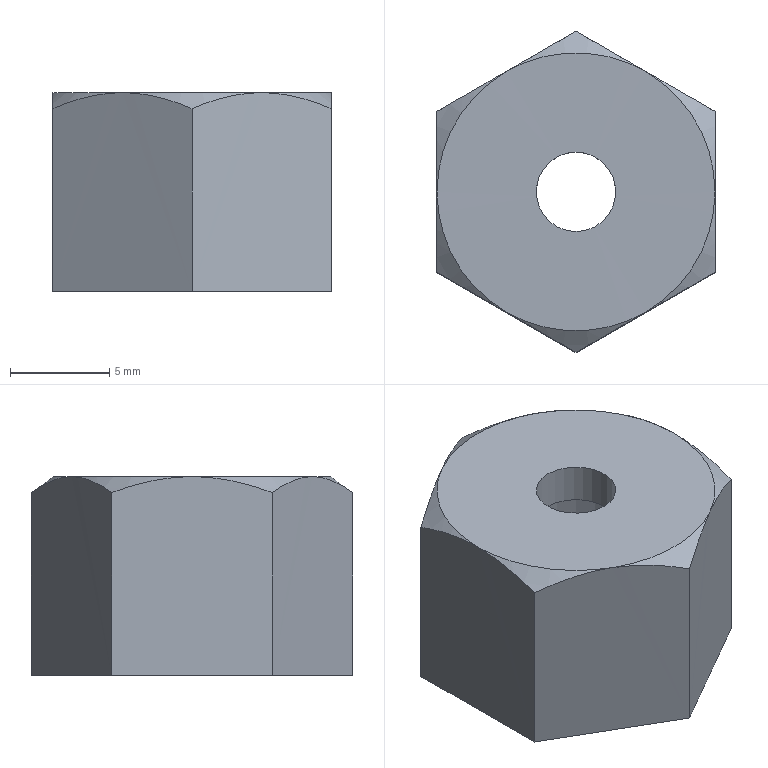Part | STEP file | 1-73.3 | 1 solid | 17 faces | box 14 x 16.166 x 10 mm | volume 1039 mm3 | plane 9 | cone 6 | cylinder 2 | commonest cylinder face diameters 4 x1 10 x1